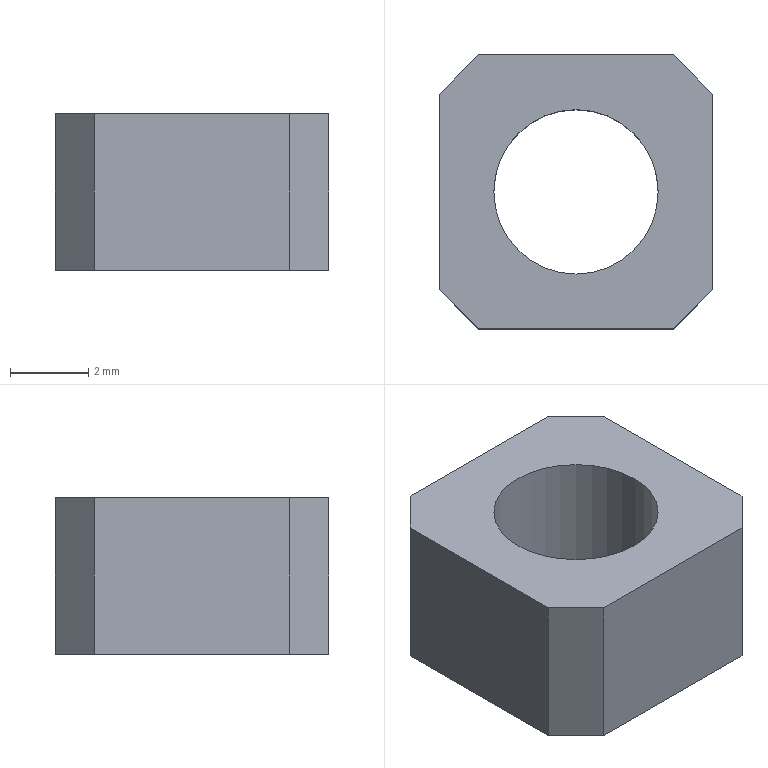Part | NX | 1 solid | 12 faces | box 7 x 7 x 4 mm | volume 132.582 mm3 | plane 10 | cylinder 2 | commonest cylinder face diameters 4.2 x2
STEP:
#1=CARTESIAN_POINT('',(6.,0.,0.));
#2=VERTEX_POINT('',#1);
#3=CARTESIAN_POINT('',(1.,0.,0.));
#4=VERTEX_POINT('',#3);
#5=CARTESIAN_POINT('',(6.,0.,0.));
#6=DIRECTION('',(-1.,0.,0.));
#7=VECTOR('',#6,1000.);
#8=LINE('',#5,#7);
#9=EDGE_CURVE('',#2,#4,#8,.T.);
#10=ORIENTED_EDGE('',*,*,#9,.T.);
#11=CARTESIAN_POINT('',(0.,1.,0.));
#12=VERTEX_POINT('',#11);
#13=CARTESIAN_POINT('',(0.,1.,0.));
#14=DIRECTION('',(0.7071,-0.7071,0.));
#15=VECTOR('',#14,1000.);
#16=LINE('',#13,#15);
#17=EDGE_CURVE('',#12,#4,#16,.T.);
#18=ORIENTED_EDGE('',*,*,#17,.F.);
#19=CARTESIAN_POINT('',(0.,6.,0.));
#20=VERTEX_POINT('',#19);
#21=CARTESIAN_POINT('',(0.,1.,0.));
#22=DIRECTION('',(0.,1.,0.));
#23=VECTOR('',#22,1000.);
#24=LINE('',#21,#23);
#25=EDGE_CURVE('',#12,#20,#24,.T.);
#26=ORIENTED_EDGE('',*,*,#25,.T.);
#27=CARTESIAN_POINT('',(1.,7.,0.));
#28=VERTEX_POINT('',#27);
#29=CARTESIAN_POINT('',(1.,7.,0.));
#30=DIRECTION('',(-0.7071,-0.7071,0.));
#31=VECTOR('',#30,1000.);
#32=LINE('',#29,#31);
#33=EDGE_CURVE('',#28,#20,#32,.T.);
#34=ORIENTED_EDGE('',*,*,#33,.F.);
#35=CARTESIAN_POINT('',(6.,7.,0.));
#36=VERTEX_POINT('',#35);
#37=CARTESIAN_POINT('',(1.,7.,0.));
#38=DIRECTION('',(1.,0.,0.));
#39=VECTOR('',#38,1000.);
#40=LINE('',#37,#39);
#41=EDGE_CURVE('',#28,#36,#40,.T.);
#42=ORIENTED_EDGE('',*,*,#41,.T.);
#43=CARTESIAN_POINT('',(7.,6.,0.));
#44=VERTEX_POINT('',#43);
#45=CARTESIAN_POINT('',(7.,6.,0.));
#46=DIRECTION('',(-0.7071,0.7071,0.));
#47=VECTOR('',#46,1000.);
#48=LINE('',#45,#47);
#49=EDGE_CURVE('',#44,#36,#48,.T.);
#50=ORIENTED_EDGE('',*,*,#49,.F.);
#51=CARTESIAN_POINT('',(7.,1.,0.));
#52=VERTEX_POINT('',#51);
#53=CARTESIAN_POINT('',(7.,6.,0.));
#54=DIRECTION('',(0.,-1.,0.));
#55=VECTOR('',#54,1000.);
#56=LINE('',#53,#55);
#57=EDGE_CURVE('',#44,#52,#56,.T.);
#58=ORIENTED_EDGE('',*,*,#57,.T.);
#59=CARTESIAN_POINT('',(6.,0.,0.));
#60=DIRECTION('',(0.7071,0.7071,0.));
#61=VECTOR('',#60,1000.);
#62=LINE('',#59,#61);
#63=EDGE_CURVE('',#2,#52,#62,.T.);
#64=ORIENTED_EDGE('',*,*,#63,.F.);
#65=EDGE_LOOP('',(#10,#18,#26,#34,#42,#50,#58,#64));
#66=FACE_BOUND('',#65,.T.);
#67=CARTESIAN_POINT('',(5.6,3.5,0.));
#68=VERTEX_POINT('',#67);
#69=CARTESIAN_POINT('',(1.4,3.5,0.));
#70=VERTEX_POINT('',#69);
#71=CARTESIAN_POINT('',(3.5,3.5,0.));
#72=DIRECTION('',(0.,0.,-1.));
#73=DIRECTION('',(-1.,0.,0.));
#74=AXIS2_PLACEMENT_3D('',#71,#72,#73);
#75=CIRCLE('',#74,2.1);
#76=EDGE_CURVE('',#68,#70,#75,.T.);
#77=ORIENTED_EDGE('',*,*,#76,.F.);
#78=CARTESIAN_POINT('',(3.5,3.5,0.));
#79=DIRECTION('',(0.,0.,-1.));
#80=DIRECTION('',(-1.,0.,0.));
#81=AXIS2_PLACEMENT_3D('',#78,#79,#80);
#82=CIRCLE('',#81,2.1);
#83=EDGE_CURVE('',#70,#68,#82,.T.);
#84=ORIENTED_EDGE('',*,*,#83,.F.);
#85=EDGE_LOOP('',(#77,#84));
#86=FACE_BOUND('',#85,.T.);
#87=CARTESIAN_POINT('',(0.,0.,0.));
#88=DIRECTION('',(0.,0.,1.));
#89=DIRECTION('',(1.,0.,0.));
#90=AXIS2_PLACEMENT_3D('',#87,#88,#89);
#91=PLANE('',#90);
#92=ADVANCED_FACE('',(#66,#86),#91,.F.);
#93=ORIENTED_EDGE('',*,*,#9,.F.);
#94=CARTESIAN_POINT('',(6.,0.,4.));
#95=VERTEX_POINT('',#94);
#96=CARTESIAN_POINT('',(6.,0.,4.));
#97=DIRECTION('',(0.,0.,-1.));
#98=VECTOR('',#97,1000.);
#99=LINE('',#96,#98);
#100=EDGE_CURVE('',#95,#2,#99,.T.);
#101=ORIENTED_EDGE('',*,*,#100,.F.);
#102=CARTESIAN_POINT('',(1.,0.,4.));
#103=VERTEX_POINT('',#102);
#104=CARTESIAN_POINT('',(6.,0.,4.));
#105=DIRECTION('',(-1.,0.,0.));
#106=VECTOR('',#105,1000.);
#107=LINE('',#104,#106);
#108=EDGE_CURVE('',#95,#103,#107,.T.);
#109=ORIENTED_EDGE('',*,*,#108,.T.);
#110=CARTESIAN_POINT('',(1.,0.,4.));
#111=DIRECTION('',(0.,0.,-1.));
#112=VECTOR('',#111,1000.);
#113=LINE('',#110,#112);
#114=EDGE_CURVE('',#103,#4,#113,.T.);
#115=ORIENTED_EDGE('',*,*,#114,.T.);
#116=EDGE_LOOP('',(#93,#101,#109,#115));
#117=FACE_BOUND('',#116,.T.);
#118=CARTESIAN_POINT('',(0.,0.,0.));
#119=DIRECTION('',(0.,-1.,0.));
#120=DIRECTION('',(0.,0.,-1.));
#121=AXIS2_PLACEMENT_3D('',#118,#119,#120);
#122=PLANE('',#121);
#123=ADVANCED_FACE('',(#117),#122,.T.);
#124=ORIENTED_EDGE('',*,*,#114,.F.);
#125=CARTESIAN_POINT('',(0.,1.,4.));
#126=VERTEX_POINT('',#125);
#127=CARTESIAN_POINT('',(1.,0.,4.));
#128=DIRECTION('',(-0.7071,0.7071,0.));
#129=VECTOR('',#128,1000.);
#130=LINE('',#127,#129);
#131=EDGE_CURVE('',#103,#126,#130,.T.);
#132=ORIENTED_EDGE('',*,*,#131,.T.);
#133=CARTESIAN_POINT('',(0.,1.,4.));
#134=DIRECTION('',(0.,0.,-1.));
#135=VECTOR('',#134,1000.);
#136=LINE('',#133,#135);
#137=EDGE_CURVE('',#126,#12,#136,.T.);
#138=ORIENTED_EDGE('',*,*,#137,.T.);
#139=ORIENTED_EDGE('',*,*,#17,.T.);
#140=EDGE_LOOP('',(#124,#132,#138,#139));
#141=FACE_BOUND('',#140,.T.);
#142=CARTESIAN_POINT('',(1.,0.,0.));
#143=DIRECTION('',(-0.7071,-0.7071,0.));
#144=DIRECTION('',(-0.7071,0.7071,0.));
#145=AXIS2_PLACEMENT_3D('',#142,#143,#144);
#146=PLANE('',#145);
#147=ADVANCED_FACE('',(#141),#146,.T.);
#148=ORIENTED_EDGE('',*,*,#25,.F.);
#149=ORIENTED_EDGE('',*,*,#137,.F.);
#150=CARTESIAN_POINT('',(0.,6.,4.));
#151=VERTEX_POINT('',#150);
#152=CARTESIAN_POINT('',(0.,1.,4.));
#153=DIRECTION('',(0.,1.,0.));
#154=VECTOR('',#153,1000.);
#155=LINE('',#152,#154);
#156=EDGE_CURVE('',#126,#151,#155,.T.);
#157=ORIENTED_EDGE('',*,*,#156,.T.);
#158=CARTESIAN_POINT('',(0.,6.,4.));
#159=DIRECTION('',(0.,0.,-1.));
#160=VECTOR('',#159,1000.);
#161=LINE('',#158,#160);
#162=EDGE_CURVE('',#151,#20,#161,.T.);
#163=ORIENTED_EDGE('',*,*,#162,.T.);
#164=EDGE_LOOP('',(#148,#149,#157,#163));
#165=FACE_BOUND('',#164,.T.);
#166=CARTESIAN_POINT('',(0.,7.,0.));
#167=DIRECTION('',(-1.,0.,0.));
#168=DIRECTION('',(0.,0.,1.));
#169=AXIS2_PLACEMENT_3D('',#166,#167,#168);
#170=PLANE('',#169);
#171=ADVANCED_FACE('',(#165),#170,.T.);
#172=ORIENTED_EDGE('',*,*,#162,.F.);
#173=CARTESIAN_POINT('',(1.,7.,4.));
#174=VERTEX_POINT('',#173);
#175=CARTESIAN_POINT('',(0.,6.,4.));
#176=DIRECTION('',(0.7071,0.7071,0.));
#177=VECTOR('',#176,1000.);
#178=LINE('',#175,#177);
#179=EDGE_CURVE('',#151,#174,#178,.T.);
#180=ORIENTED_EDGE('',*,*,#179,.T.);
#181=CARTESIAN_POINT('',(1.,7.,4.));
#182=DIRECTION('',(0.,0.,-1.));
#183=VECTOR('',#182,1000.);
#184=LINE('',#181,#183);
#185=EDGE_CURVE('',#174,#28,#184,.T.);
#186=ORIENTED_EDGE('',*,*,#185,.T.);
#187=ORIENTED_EDGE('',*,*,#33,.T.);
#188=EDGE_LOOP('',(#172,#180,#186,#187));
#189=FACE_BOUND('',#188,.T.);
#190=CARTESIAN_POINT('',(0.,6.,0.));
#191=DIRECTION('',(-0.7071,0.7071,0.));
#192=DIRECTION('',(0.,0.,1.));
#193=AXIS2_PLACEMENT_3D('',#190,#191,#192);
#194=PLANE('',#193);
#195=ADVANCED_FACE('',(#189),#194,.T.);
#196=ORIENTED_EDGE('',*,*,#41,.F.);
#197=ORIENTED_EDGE('',*,*,#185,.F.);
#198=CARTESIAN_POINT('',(6.,7.,4.));
#199=VERTEX_POINT('',#198);
#200=CARTESIAN_POINT('',(1.,7.,4.));
#201=DIRECTION('',(1.,0.,0.));
#202=VECTOR('',#201,1000.);
#203=LINE('',#200,#202);
#204=EDGE_CURVE('',#174,#199,#203,.T.);
#205=ORIENTED_EDGE('',*,*,#204,.T.);
#206=CARTESIAN_POINT('',(6.,7.,4.));
#207=DIRECTION('',(0.,0.,-1.));
#208=VECTOR('',#207,1000.);
#209=LINE('',#206,#208);
#210=EDGE_CURVE('',#199,#36,#209,.T.);
#211=ORIENTED_EDGE('',*,*,#210,.T.);
#212=EDGE_LOOP('',(#196,#197,#205,#211));
#213=FACE_BOUND('',#212,.T.);
#214=CARTESIAN_POINT('',(7.,7.,0.));
#215=DIRECTION('',(0.,1.,0.));
#216=DIRECTION('',(1.,0.,0.));
#217=AXIS2_PLACEMENT_3D('',#214,#215,#216);
#218=PLANE('',#217);
#219=ADVANCED_FACE('',(#213),#218,.T.);
#220=ORIENTED_EDGE('',*,*,#210,.F.);
#221=CARTESIAN_POINT('',(7.,6.,4.));
#222=VERTEX_POINT('',#221);
#223=CARTESIAN_POINT('',(6.,7.,4.));
#224=DIRECTION('',(0.7071,-0.7071,0.));
#225=VECTOR('',#224,1000.);
#226=LINE('',#223,#225);
#227=EDGE_CURVE('',#199,#222,#226,.T.);
#228=ORIENTED_EDGE('',*,*,#227,.T.);
#229=CARTESIAN_POINT('',(7.,6.,4.));
#230=DIRECTION('',(0.,0.,-1.));
#231=VECTOR('',#230,1000.);
#232=LINE('',#229,#231);
#233=EDGE_CURVE('',#222,#44,#232,.T.);
#234=ORIENTED_EDGE('',*,*,#233,.T.);
#235=ORIENTED_EDGE('',*,*,#49,.T.);
#236=EDGE_LOOP('',(#220,#228,#234,#235));
#237=FACE_BOUND('',#236,.T.);
#238=CARTESIAN_POINT('',(6.,7.,0.));
#239=DIRECTION('',(0.7071,0.7071,0.));
#240=DIRECTION('',(0.,0.,-1.));
#241=AXIS2_PLACEMENT_3D('',#238,#239,#240);
#242=PLANE('',#241);
#243=ADVANCED_FACE('',(#237),#242,.T.);
#244=ORIENTED_EDGE('',*,*,#57,.F.);
#245=ORIENTED_EDGE('',*,*,#233,.F.);
#246=CARTESIAN_POINT('',(7.,1.,4.));
#247=VERTEX_POINT('',#246);
#248=CARTESIAN_POINT('',(7.,6.,4.));
#249=DIRECTION('',(0.,-1.,0.));
#250=VECTOR('',#249,1000.);
#251=LINE('',#248,#250);
#252=EDGE_CURVE('',#222,#247,#251,.T.);
#253=ORIENTED_EDGE('',*,*,#252,.T.);
#254=CARTESIAN_POINT('',(7.,1.,4.));
#255=DIRECTION('',(0.,0.,-1.));
#256=VECTOR('',#255,1000.);
#257=LINE('',#254,#256);
#258=EDGE_CURVE('',#247,#52,#257,.T.);
#259=ORIENTED_EDGE('',*,*,#258,.T.);
#260=EDGE_LOOP('',(#244,#245,#253,#259));
#261=FACE_BOUND('',#260,.T.);
#262=CARTESIAN_POINT('',(7.,0.,0.));
#263=DIRECTION('',(1.,0.,0.));
#264=DIRECTION('',(0.,1.,0.));
#265=AXIS2_PLACEMENT_3D('',#262,#263,#264);
#266=PLANE('',#265);
#267=ADVANCED_FACE('',(#261),#266,.T.);
#268=ORIENTED_EDGE('',*,*,#258,.F.);
#269=CARTESIAN_POINT('',(7.,1.,4.));
#270=DIRECTION('',(-0.7071,-0.7071,0.));
#271=VECTOR('',#270,1000.);
#272=LINE('',#269,#271);
#273=EDGE_CURVE('',#247,#95,#272,.T.);
#274=ORIENTED_EDGE('',*,*,#273,.T.);
#275=ORIENTED_EDGE('',*,*,#100,.T.);
#276=ORIENTED_EDGE('',*,*,#63,.T.);
#277=EDGE_LOOP('',(#268,#274,#275,#276));
#278=FACE_BOUND('',#277,.T.);
#279=CARTESIAN_POINT('',(7.,1.,0.));
#280=DIRECTION('',(0.7071,-0.7071,0.));
#281=DIRECTION('',(0.,0.,-1.));
#282=AXIS2_PLACEMENT_3D('',#279,#280,#281);
#283=PLANE('',#282);
#284=ADVANCED_FACE('',(#278),#283,.T.);
#285=ORIENTED_EDGE('',*,*,#108,.F.);
#286=ORIENTED_EDGE('',*,*,#273,.F.);
#287=ORIENTED_EDGE('',*,*,#252,.F.);
#288=ORIENTED_EDGE('',*,*,#227,.F.);
#289=ORIENTED_EDGE('',*,*,#204,.F.);
#290=ORIENTED_EDGE('',*,*,#179,.F.);
#291=ORIENTED_EDGE('',*,*,#156,.F.);
#292=ORIENTED_EDGE('',*,*,#131,.F.);
#293=EDGE_LOOP('',(#285,#286,#287,#288,#289,#290,#291,#292));
#294=FACE_BOUND('',#293,.T.);
#295=CARTESIAN_POINT('',(5.6,3.5,4.));
#296=VERTEX_POINT('',#295);
#297=CARTESIAN_POINT('',(1.4,3.5,4.));
#298=VERTEX_POINT('',#297);
#299=CARTESIAN_POINT('',(3.5,3.5,4.));
#300=DIRECTION('',(0.,0.,1.));
#301=DIRECTION('',(1.,0.,0.));
#302=AXIS2_PLACEMENT_3D('',#299,#300,#301);
#303=CIRCLE('',#302,2.1);
#304=EDGE_CURVE('',#296,#298,#303,.T.);
#305=ORIENTED_EDGE('',*,*,#304,.F.);
#306=CARTESIAN_POINT('',(3.5,3.5,4.));
#307=DIRECTION('',(0.,0.,1.));
#308=DIRECTION('',(1.,0.,0.));
#309=AXIS2_PLACEMENT_3D('',#306,#307,#308);
#310=CIRCLE('',#309,2.1);
#311=EDGE_CURVE('',#298,#296,#310,.T.);
#312=ORIENTED_EDGE('',*,*,#311,.F.);
#313=EDGE_LOOP('',(#305,#312));
#314=FACE_BOUND('',#313,.T.);
#315=CARTESIAN_POINT('',(0.,0.,4.));
#316=DIRECTION('',(0.,0.,1.));
#317=DIRECTION('',(1.,0.,0.));
#318=AXIS2_PLACEMENT_3D('',#315,#316,#317);
#319=PLANE('',#318);
#320=ADVANCED_FACE('',(#294,#314),#319,.T.);
#321=ORIENTED_EDGE('',*,*,#76,.T.);
#322=CARTESIAN_POINT('',(1.4,3.5,-0.675));
#323=DIRECTION('',(0.,0.,1.));
#324=VECTOR('',#323,1000.);
#325=LINE('',#322,#324);
#326=EDGE_CURVE('',#298,#70,#325,.F.);
#327=ORIENTED_EDGE('',*,*,#326,.F.);
#328=ORIENTED_EDGE('',*,*,#311,.T.);
#329=CARTESIAN_POINT('',(5.6,3.5,-0.675));
#330=DIRECTION('',(0.,0.,1.));
#331=VECTOR('',#330,1000.);
#332=LINE('',#329,#331);
#333=EDGE_CURVE('',#296,#68,#332,.F.);
#334=ORIENTED_EDGE('',*,*,#333,.T.);
#335=EDGE_LOOP('',(#321,#327,#328,#334));
#336=FACE_BOUND('',#335,.T.);
#337=CARTESIAN_POINT('',(3.5,3.5,-0.675));
#338=DIRECTION('',(0.,0.,1.));
#339=DIRECTION('',(-1.,0.,0.));
#340=AXIS2_PLACEMENT_3D('',#337,#338,#339);
#341=CYLINDRICAL_SURFACE('',#340,2.1);
#342=ADVANCED_FACE('',(#336),#341,.F.);
#343=ORIENTED_EDGE('',*,*,#304,.T.);
#344=ORIENTED_EDGE('',*,*,#326,.T.);
#345=ORIENTED_EDGE('',*,*,#83,.T.);
#346=ORIENTED_EDGE('',*,*,#333,.F.);
#347=EDGE_LOOP('',(#343,#344,#345,#346));
#348=FACE_BOUND('',#347,.T.);
#349=CARTESIAN_POINT('',(3.5,3.5,-0.675));
#350=DIRECTION('',(0.,0.,1.));
#351=DIRECTION('',(-1.,0.,0.));
#352=AXIS2_PLACEMENT_3D('',#349,#350,#351);
#353=CYLINDRICAL_SURFACE('',#352,2.1);
#354=ADVANCED_FACE('',(#348),#353,.F.);
#355=CLOSED_SHELL('',(#92,#123,#147,#171,#195,#219,#243,#267,#284,#320,#342,#354));
#356=MANIFOLD_SOLID_BREP('',#355);
#357=(LENGTH_UNIT()NAMED_UNIT(*)SI_UNIT(.MILLI.,.METRE.));
#358=UNCERTAINTY_MEASURE_WITH_UNIT(LENGTH_MEASURE(0.00001),#357,'','');
#359=(NAMED_UNIT(*)PLANE_ANGLE_UNIT()SI_UNIT($,.RADIAN.));
#360=(NAMED_UNIT(*)SI_UNIT($,.STERADIAN.)SOLID_ANGLE_UNIT());
#361=(GEOMETRIC_REPRESENTATION_CONTEXT(3)GLOBAL_UNCERTAINTY_ASSIGNED_CONTEXT((#358))GLOBAL_UNIT_ASSIGNED_CONTEXT((#357,#359,#360))REPRESENTATION_CONTEXT('',''));
#362=ADVANCED_BREP_SHAPE_REPRESENTATION('',(#356),#361);